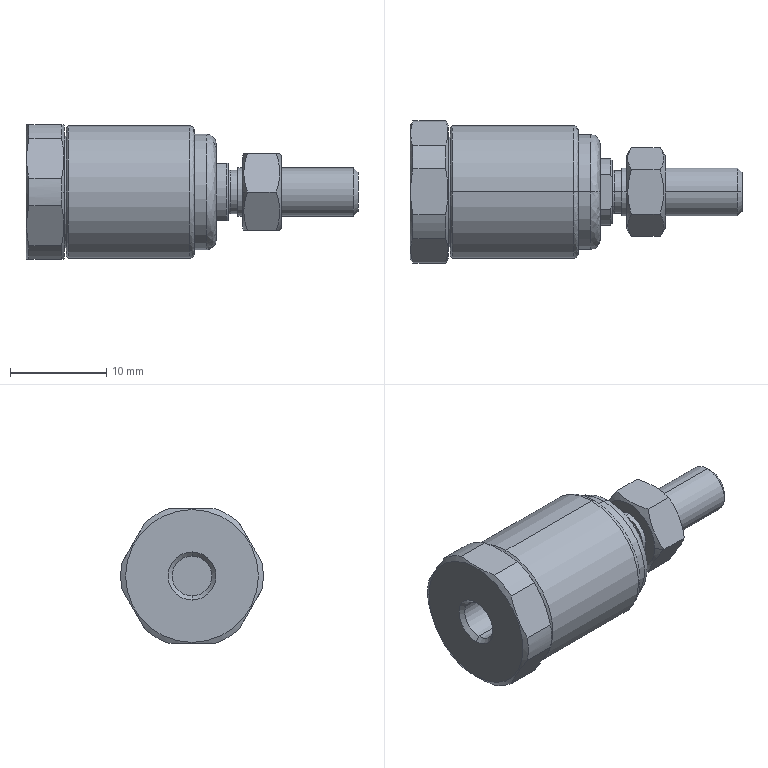Part | STEP file | F-M5X080F | 1 solid | 75 faces | box 34.5 x 14.8 x 14 mm | volume 3243 mm3 | plane 27 | cylinder 22 | cone 18 | spline 8 | commonest cylinder face diameters 14.8 x6 5 x4 4.134 x2 4.5 x2 7 x2 11.6 x2